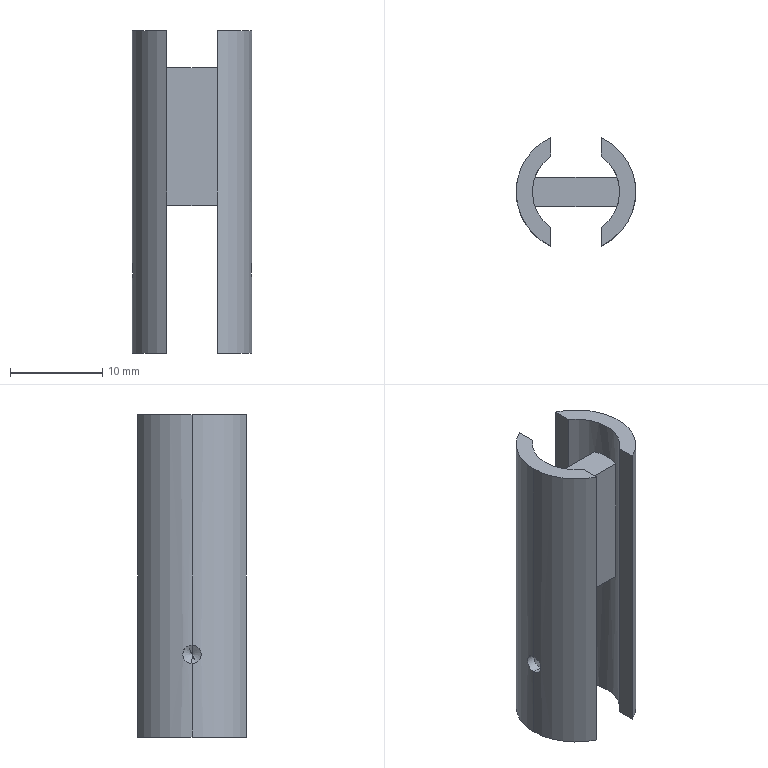Part | STEP file | magnetizing head 3 | 1 solid | 26 faces | box 13 x 11.779 x 35 mm | volume 1900 mm3 | plane 12 | cylinder 10 | cone 4 | commonest cylinder face diameters 2 x4 9.5 x3 13 x3